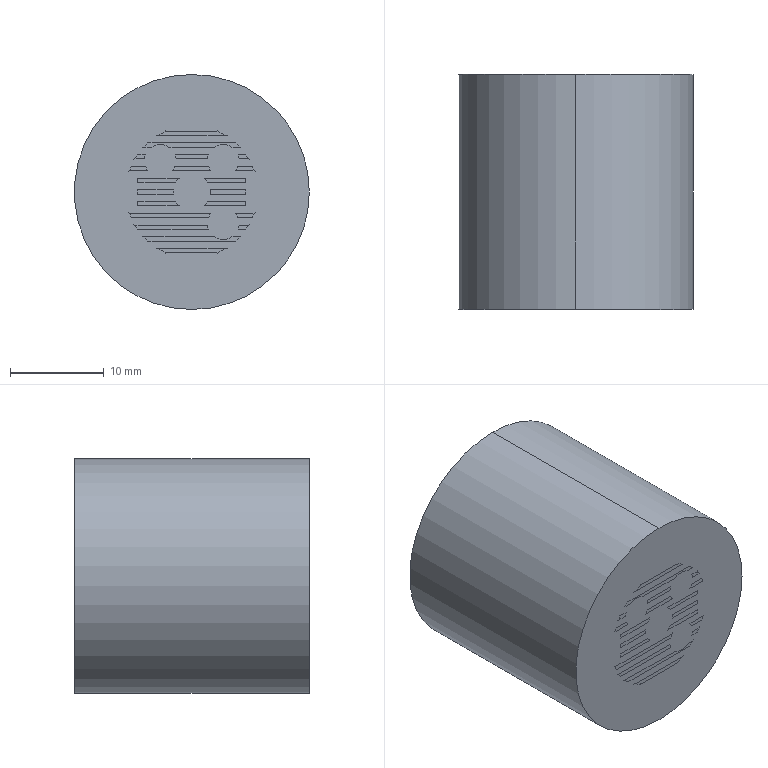Part | 2 solids | 138 faces | box 25 x 25 x 25 mm | volume 14029 mm3 | plane 97 | cylinder 36 | cone 5 | commonest cylinder face diameters 5.5 x7 3.4 x6 2 x2 2.16 x2 3.5 x2 4 x2